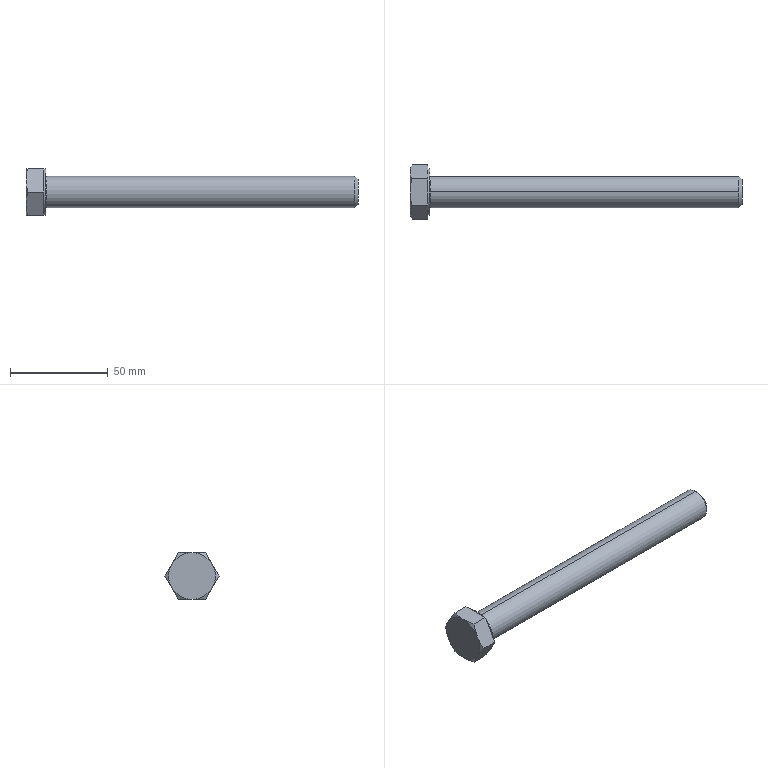Part | SolidWorks | features RevCut 4, Chamfer 1, Extrusion 1, Fillet 1, LPattern 1, Revolution 1 | 1 solid | 35 faces | box 170 x 27.713 x 24 mm | volume 37050 mm3 | plane 15 | cone 14 | cylinder 4 | torus 2 | commonest cylinder face diameters 16 x2 24 x2
STEP:
#1=CARTESIAN_POINT('',(10.6,0.,8.));
#2=VERTEX_POINT('',#1);
#3=CARTESIAN_POINT('',(10.6,0.,-8.));
#4=VERTEX_POINT('',#3);
#5=CARTESIAN_POINT('',(10.6,0.,0.));
#6=DIRECTION('',(1.,0.,0.));
#7=DIRECTION('',(0.,0.,-1.));
#8=AXIS2_PLACEMENT_3D('',#5,#6,#7);
#9=CIRCLE('',#8,8.);
#10=EDGE_CURVE('',#2,#4,#9,.T.);
#11=ORIENTED_EDGE('',*,*,#10,.F.);
#12=CARTESIAN_POINT('',(10.,0.,8.6));
#13=VERTEX_POINT('',#12);
#14=CARTESIAN_POINT('',(10.6,0.,8.6));
#15=DIRECTION('',(0.,1.,0.));
#16=DIRECTION('',(0.,0.,1.));
#17=AXIS2_PLACEMENT_3D('',#14,#15,#16);
#18=CIRCLE('',#17,0.6);
#19=EDGE_CURVE('',#2,#13,#18,.T.);
#20=ORIENTED_EDGE('',*,*,#19,.T.);
#21=CARTESIAN_POINT('',(10.,0.,-8.6));
#22=VERTEX_POINT('',#21);
#23=CARTESIAN_POINT('',(10.,0.,0.));
#24=DIRECTION('',(-1.,0.,0.));
#25=DIRECTION('',(0.,0.,-1.));
#26=AXIS2_PLACEMENT_3D('',#23,#24,#25);
#27=CIRCLE('',#26,8.6);
#28=EDGE_CURVE('',#22,#13,#27,.T.);
#29=ORIENTED_EDGE('',*,*,#28,.F.);
#30=CARTESIAN_POINT('',(10.6,0.,-8.6));
#31=DIRECTION('',(0.,-1.,0.));
#32=DIRECTION('',(0.,0.,-1.));
#33=AXIS2_PLACEMENT_3D('',#30,#31,#32);
#34=CIRCLE('',#33,0.6);
#35=EDGE_CURVE('',#4,#22,#34,.T.);
#36=ORIENTED_EDGE('',*,*,#35,.F.);
#37=EDGE_LOOP('',(#11,#20,#29,#36));
#38=FACE_OUTER_BOUND('',#37,.T.);
#39=CARTESIAN_POINT('',(10.6,0.,0.));
#40=DIRECTION('',(1.,0.,0.));
#41=DIRECTION('',(0.,0.,-1.));
#42=AXIS2_PLACEMENT_3D('',#39,#40,#41);
#43=TOROIDAL_SURFACE('',#42,8.6,0.6);
#44=ADVANCED_FACE('',(#38),#43,.F.);
#45=CARTESIAN_POINT('',(170.,0.,-6.4));
#46=VERTEX_POINT('',#45);
#47=CARTESIAN_POINT('',(170.,0.,6.4));
#48=VERTEX_POINT('',#47);
#49=CARTESIAN_POINT('',(170.,0.,0.));
#50=DIRECTION('',(1.,0.,0.));
#51=DIRECTION('',(0.,0.,1.));
#52=AXIS2_PLACEMENT_3D('',#49,#50,#51);
#53=CIRCLE('',#52,6.4);
#54=EDGE_CURVE('',#46,#48,#53,.T.);
#55=ORIENTED_EDGE('',*,*,#54,.F.);
#56=CARTESIAN_POINT('',(168.4,0.,-8.));
#57=VERTEX_POINT('',#56);
#58=CARTESIAN_POINT('',(168.4,0.,-8.));
#59=DIRECTION('',(-0.7071,0.,-0.7071));
#60=VECTOR('',#59,1000.);
#61=LINE('',#58,#60);
#62=EDGE_CURVE('',#46,#57,#61,.T.);
#63=ORIENTED_EDGE('',*,*,#62,.T.);
#64=CARTESIAN_POINT('',(168.4,0.,8.));
#65=VERTEX_POINT('',#64);
#66=CARTESIAN_POINT('',(168.4,0.,0.));
#67=DIRECTION('',(-1.,0.,0.));
#68=DIRECTION('',(0.,0.,1.));
#69=AXIS2_PLACEMENT_3D('',#66,#67,#68);
#70=CIRCLE('',#69,8.);
#71=EDGE_CURVE('',#65,#57,#70,.T.);
#72=ORIENTED_EDGE('',*,*,#71,.F.);
#73=CARTESIAN_POINT('',(168.4,0.,8.));
#74=DIRECTION('',(-0.7071,0.,0.7071));
#75=VECTOR('',#74,1000.);
#76=LINE('',#73,#75);
#77=EDGE_CURVE('',#48,#65,#76,.T.);
#78=ORIENTED_EDGE('',*,*,#77,.F.);
#79=EDGE_LOOP('',(#55,#63,#72,#78));
#80=FACE_OUTER_BOUND('',#79,.T.);
#81=CARTESIAN_POINT('',(168.4,0.,0.));
#82=DIRECTION('',(-1.,0.,0.));
#83=DIRECTION('',(0.,0.,1.));
#84=AXIS2_PLACEMENT_3D('',#81,#82,#83);
#85=CONICAL_SURFACE('',#84,8.,0.7854);
#86=ADVANCED_FACE('',(#80),#85,.T.);
#87=ORIENTED_EDGE('',*,*,#71,.T.);
#88=CARTESIAN_POINT('',(0.,0.,-8.));
#89=DIRECTION('',(-1.,0.,0.));
#90=VECTOR('',#89,1000.);
#91=LINE('',#88,#90);
#92=EDGE_CURVE('',#57,#4,#91,.T.);
#93=ORIENTED_EDGE('',*,*,#92,.T.);
#94=CARTESIAN_POINT('',(10.6,0.,0.));
#95=DIRECTION('',(1.,0.,0.));
#96=DIRECTION('',(0.,0.,-1.));
#97=AXIS2_PLACEMENT_3D('',#94,#95,#96);
#98=CIRCLE('',#97,8.);
#99=EDGE_CURVE('',#4,#2,#98,.T.);
#100=ORIENTED_EDGE('',*,*,#99,.T.);
#101=CARTESIAN_POINT('',(0.,0.,8.));
#102=DIRECTION('',(-1.,0.,0.));
#103=VECTOR('',#102,1000.);
#104=LINE('',#101,#103);
#105=EDGE_CURVE('',#65,#2,#104,.T.);
#106=ORIENTED_EDGE('',*,*,#105,.F.);
#107=EDGE_LOOP('',(#87,#93,#100,#106));
#108=FACE_OUTER_BOUND('',#107,.T.);
#109=CARTESIAN_POINT('',(0.,0.,0.));
#110=DIRECTION('',(-1.,0.,0.));
#111=DIRECTION('',(0.,0.,1.));
#112=AXIS2_PLACEMENT_3D('',#109,#110,#111);
#113=CYLINDRICAL_SURFACE('',#112,8.);
#114=ADVANCED_FACE('',(#108),#113,.T.);
#115=CARTESIAN_POINT('',(10.,0.,-12.));
#116=VERTEX_POINT('',#115);
#117=CARTESIAN_POINT('',(10.,0.,12.));
#118=VERTEX_POINT('',#117);
#119=CARTESIAN_POINT('',(10.,0.,0.));
#120=DIRECTION('',(1.,0.,0.));
#121=DIRECTION('',(0.,0.,-1.));
#122=AXIS2_PLACEMENT_3D('',#119,#120,#121);
#123=CIRCLE('',#122,12.);
#124=EDGE_CURVE('',#116,#118,#123,.T.);
#125=ORIENTED_EDGE('',*,*,#124,.F.);
#126=CARTESIAN_POINT('',(9.2,0.,-12.));
#127=VERTEX_POINT('',#126);
#128=CARTESIAN_POINT('',(0.,0.,-12.));
#129=DIRECTION('',(-1.,0.,0.));
#130=VECTOR('',#129,1000.);
#131=LINE('',#128,#130);
#132=EDGE_CURVE('',#116,#127,#131,.T.);
#133=ORIENTED_EDGE('',*,*,#132,.T.);
#134=CARTESIAN_POINT('',(9.2,10.392,-6.));
#135=VERTEX_POINT('',#134);
#136=CARTESIAN_POINT('',(9.2,0.,0.));
#137=DIRECTION('',(-1.,0.,0.));
#138=DIRECTION('',(0.,0.,1.));
#139=AXIS2_PLACEMENT_3D('',#136,#137,#138);
#140=CIRCLE('',#139,12.);
#141=EDGE_CURVE('',#135,#127,#140,.T.);
#142=ORIENTED_EDGE('',*,*,#141,.F.);
#143=CARTESIAN_POINT('',(9.2,10.392,6.));
#144=VERTEX_POINT('',#143);
#145=CARTESIAN_POINT('',(9.2,0.,0.));
#146=DIRECTION('',(-1.,0.,0.));
#147=DIRECTION('',(0.,0.,1.));
#148=AXIS2_PLACEMENT_3D('',#145,#146,#147);
#149=CIRCLE('',#148,12.);
#150=EDGE_CURVE('',#144,#135,#149,.T.);
#151=ORIENTED_EDGE('',*,*,#150,.F.);
#152=CARTESIAN_POINT('',(9.2,0.,12.));
#153=VERTEX_POINT('',#152);
#154=CARTESIAN_POINT('',(9.2,0.,0.));
#155=DIRECTION('',(-1.,0.,0.));
#156=DIRECTION('',(0.,0.,1.));
#157=AXIS2_PLACEMENT_3D('',#154,#155,#156);
#158=CIRCLE('',#157,12.);
#159=EDGE_CURVE('',#153,#144,#158,.T.);
#160=ORIENTED_EDGE('',*,*,#159,.F.);
#161=CARTESIAN_POINT('',(0.,0.,12.));
#162=DIRECTION('',(-1.,0.,0.));
#163=VECTOR('',#162,1000.);
#164=LINE('',#161,#163);
#165=EDGE_CURVE('',#118,#153,#164,.T.);
#166=ORIENTED_EDGE('',*,*,#165,.F.);
#167=EDGE_LOOP('',(#125,#133,#142,#151,#160,#166));
#168=FACE_OUTER_BOUND('',#167,.T.);
#169=CARTESIAN_POINT('',(0.,0.,0.));
#170=DIRECTION('',(-1.,0.,0.));
#171=DIRECTION('',(0.,0.,1.));
#172=AXIS2_PLACEMENT_3D('',#169,#170,#171);
#173=CYLINDRICAL_SURFACE('',#172,12.);
#174=ADVANCED_FACE('',(#168),#173,.T.);
#175=CARTESIAN_POINT('',(9.2,7.427,-11.136));
#176=VERTEX_POINT('',#175);
#177=CARTESIAN_POINT('',(9.2,6.928,-12.));
#178=DIRECTION('',(0.,0.5,0.866));
#179=VECTOR('',#178,1000.);
#180=LINE('',#177,#179);
#181=EDGE_CURVE('',#176,#135,#180,.T.);
#182=ORIENTED_EDGE('',*,*,#181,.F.);
#183=CARTESIAN_POINT('',(8.928,6.928,-12.));
#184=VERTEX_POINT('',#183);
#185=CARTESIAN_POINT('',(8.928,6.928,-12.));
#186=CARTESIAN_POINT('',(9.024,7.094,-11.713));
#187=CARTESIAN_POINT('',(9.115,7.26,-11.425));
#188=CARTESIAN_POINT('',(9.2,7.427,-11.136));
#189=B_SPLINE_CURVE_WITH_KNOTS('',3,(#185,#186,#187,#188),.UNSPECIFIED.,.F.,.F.,(4,4),(0.000000238,0.001026),.UNSPECIFIED.);
#190=EDGE_CURVE('',#184,#176,#189,.T.);
#191=ORIENTED_EDGE('',*,*,#190,.F.);
#192=CARTESIAN_POINT('',(1.072,6.928,-12.));
#193=VERTEX_POINT('',#192);
#194=CARTESIAN_POINT('',(10.,6.928,-12.));
#195=DIRECTION('',(-1.,0.,0.));
#196=VECTOR('',#195,1000.);
#197=LINE('',#194,#196);
#198=EDGE_CURVE('',#184,#193,#197,.T.);
#199=ORIENTED_EDGE('',*,*,#198,.T.);
#200=CARTESIAN_POINT('',(0.,10.392,-6.));
#201=VERTEX_POINT('',#200);
#202=CARTESIAN_POINT('',(0.,10.392,-6.));
#203=CARTESIAN_POINT('',(0.,10.098,-6.509));
#204=CARTESIAN_POINT('',(0.02533,9.803,-7.021));
#205=CARTESIAN_POINT('',(0.1234,9.219,-8.033));
#206=CARTESIAN_POINT('',(0.196,8.929,-8.535));
#207=CARTESIAN_POINT('',(0.476,8.063,-10.034));
#208=CARTESIAN_POINT('',(0.7454,7.493,-11.021));
#209=CARTESIAN_POINT('',(1.072,6.928,-12.));
#210=B_SPLINE_CURVE_WITH_KNOTS('',3,(#202,#203,#204,#205,#206,#207,#208,#209),.UNSPECIFIED.,.F.,.F.,(4,2,2,4),(0.00701,0.008756,0.0105,0.01399),.UNSPECIFIED.);
#211=EDGE_CURVE('',#201,#193,#210,.T.);
#212=ORIENTED_EDGE('',*,*,#211,.F.);
#213=CARTESIAN_POINT('',(1.072,13.856,0.));
#214=VERTEX_POINT('',#213);
#215=CARTESIAN_POINT('',(1.072,13.856,0.));
#216=CARTESIAN_POINT('',(0.7446,13.29,-0.9815));
#217=CARTESIAN_POINT('',(0.4751,12.719,-1.97));
#218=CARTESIAN_POINT('',(0.1021,11.565,-3.968));
#219=CARTESIAN_POINT('',(0.,10.982,-4.978));
#220=CARTESIAN_POINT('',(0.,10.392,-6.));
#221=B_SPLINE_CURVE_WITH_KNOTS('',3,(#215,#216,#217,#218,#219,#220),.UNSPECIFIED.,.F.,.F.,(4,2,4),(0.000000238,0.003505,0.00701),.UNSPECIFIED.);
#222=EDGE_CURVE('',#214,#201,#221,.T.);
#223=ORIENTED_EDGE('',*,*,#222,.F.);
#224=CARTESIAN_POINT('',(8.928,13.856,0.));
#225=VERTEX_POINT('',#224);
#226=CARTESIAN_POINT('',(10.,13.856,0.));
#227=DIRECTION('',(-1.,0.,0.));
#228=VECTOR('',#227,1000.);
#229=LINE('',#226,#228);
#230=EDGE_CURVE('',#225,#214,#229,.T.);
#231=ORIENTED_EDGE('',*,*,#230,.F.);
#232=CARTESIAN_POINT('',(9.2,13.358,-0.8637));
#233=VERTEX_POINT('',#232);
#234=CARTESIAN_POINT('',(9.2,13.358,-0.8637));
#235=CARTESIAN_POINT('',(9.115,13.524,-0.575));
#236=CARTESIAN_POINT('',(9.024,13.691,-0.2872));
#237=CARTESIAN_POINT('',(8.928,13.856,0.));
#238=B_SPLINE_CURVE_WITH_KNOTS('',3,(#234,#235,#236,#237),.UNSPECIFIED.,.F.,.F.,(4,4),(0.01297,0.01399),.UNSPECIFIED.);
#239=EDGE_CURVE('',#233,#225,#238,.T.);
#240=ORIENTED_EDGE('',*,*,#239,.F.);
#241=CARTESIAN_POINT('',(9.2,6.928,-12.));
#242=DIRECTION('',(0.,0.5,0.866));
#243=VECTOR('',#242,1000.);
#244=LINE('',#241,#243);
#245=EDGE_CURVE('',#135,#233,#244,.T.);
#246=ORIENTED_EDGE('',*,*,#245,.F.);
#247=EDGE_LOOP('',(#182,#191,#199,#212,#223,#231,#240,#246));
#248=FACE_OUTER_BOUND('',#247,.T.);
#249=CARTESIAN_POINT('',(10.,6.928,-12.));
#250=DIRECTION('',(0.,-0.866,0.5));
#251=DIRECTION('',(0.,-0.5,-0.866));
#252=AXIS2_PLACEMENT_3D('',#249,#250,#251);
#253=PLANE('',#252);
#254=ADVANCED_FACE('',(#248),#253,.F.);
#255=CARTESIAN_POINT('',(9.2,13.358,0.8637));
#256=VERTEX_POINT('',#255);
#257=CARTESIAN_POINT('',(9.2,13.856,0.));
#258=DIRECTION('',(0.,-0.5,0.866));
#259=VECTOR('',#258,1000.);
#260=LINE('',#257,#259);
#261=EDGE_CURVE('',#256,#144,#260,.T.);
#262=ORIENTED_EDGE('',*,*,#261,.F.);
#263=CARTESIAN_POINT('',(8.928,13.856,0.));
#264=CARTESIAN_POINT('',(9.024,13.691,0.2873));
#265=CARTESIAN_POINT('',(9.115,13.524,0.5751));
#266=CARTESIAN_POINT('',(9.2,13.358,0.8637));
#267=B_SPLINE_CURVE_WITH_KNOTS('',3,(#263,#264,#265,#266),.UNSPECIFIED.,.F.,.F.,(4,4),(0.000000238,0.001026),.UNSPECIFIED.);
#268=EDGE_CURVE('',#225,#256,#267,.T.);
#269=ORIENTED_EDGE('',*,*,#268,.F.);
#270=ORIENTED_EDGE('',*,*,#230,.T.);
#271=CARTESIAN_POINT('',(0.,10.392,6.));
#272=VERTEX_POINT('',#271);
#273=CARTESIAN_POINT('',(0.,10.392,6.));
#274=CARTESIAN_POINT('',(0.,10.686,5.491));
#275=CARTESIAN_POINT('',(0.02533,10.982,4.979));
#276=CARTESIAN_POINT('',(0.1234,11.566,3.967));
#277=CARTESIAN_POINT('',(0.196,11.856,3.465));
#278=CARTESIAN_POINT('',(0.476,12.721,1.966));
#279=CARTESIAN_POINT('',(0.7454,13.291,0.9791));
#280=CARTESIAN_POINT('',(1.072,13.856,0.));
#281=B_SPLINE_CURVE_WITH_KNOTS('',3,(#273,#274,#275,#276,#277,#278,#279,#280),.UNSPECIFIED.,.F.,.F.,(4,2,2,4),(0.00701,0.008756,0.0105,0.01399),.UNSPECIFIED.);
#282=EDGE_CURVE('',#272,#214,#281,.T.);
#283=ORIENTED_EDGE('',*,*,#282,.F.);
#284=CARTESIAN_POINT('',(1.072,6.928,12.));
#285=VERTEX_POINT('',#284);
#286=CARTESIAN_POINT('',(1.072,6.928,12.));
#287=CARTESIAN_POINT('',(0.7446,7.495,11.018));
#288=CARTESIAN_POINT('',(0.4751,8.066,10.03));
#289=CARTESIAN_POINT('',(0.1021,9.219,8.032));
#290=CARTESIAN_POINT('',(0.,9.802,7.022));
#291=CARTESIAN_POINT('',(0.,10.392,6.));
#292=B_SPLINE_CURVE_WITH_KNOTS('',3,(#286,#287,#288,#289,#290,#291),.UNSPECIFIED.,.F.,.F.,(4,2,4),(0.000000238,0.003505,0.00701),.UNSPECIFIED.);
#293=EDGE_CURVE('',#285,#272,#292,.T.);
#294=ORIENTED_EDGE('',*,*,#293,.F.);
#295=CARTESIAN_POINT('',(8.928,6.928,12.));
#296=VERTEX_POINT('',#295);
#297=CARTESIAN_POINT('',(10.,6.928,12.));
#298=DIRECTION('',(-1.,0.,0.));
#299=VECTOR('',#298,1000.);
#300=LINE('',#297,#299);
#301=EDGE_CURVE('',#296,#285,#300,.T.);
#302=ORIENTED_EDGE('',*,*,#301,.F.);
#303=CARTESIAN_POINT('',(9.2,7.427,11.136));
#304=VERTEX_POINT('',#303);
#305=CARTESIAN_POINT('',(9.2,7.427,11.136));
#306=CARTESIAN_POINT('',(9.115,7.26,11.425));
#307=CARTESIAN_POINT('',(9.024,7.094,11.713));
#308=CARTESIAN_POINT('',(8.928,6.928,12.));
#309=B_SPLINE_CURVE_WITH_KNOTS('',3,(#305,#306,#307,#308),.UNSPECIFIED.,.F.,.F.,(4,4),(0.01297,0.01399),.UNSPECIFIED.);
#310=EDGE_CURVE('',#304,#296,#309,.T.);
#311=ORIENTED_EDGE('',*,*,#310,.F.);
#312=CARTESIAN_POINT('',(9.2,13.856,0.));
#313=DIRECTION('',(0.,-0.5,0.866));
#314=VECTOR('',#313,1000.);
#315=LINE('',#312,#314);
#316=EDGE_CURVE('',#144,#304,#315,.T.);
#317=ORIENTED_EDGE('',*,*,#316,.F.);
#318=EDGE_LOOP('',(#262,#269,#270,#283,#294,#302,#311,#317));
#319=FACE_OUTER_BOUND('',#318,.T.);
#320=CARTESIAN_POINT('',(10.,13.856,0.));
#321=DIRECTION('',(0.,-0.866,-0.5));
#322=DIRECTION('',(0.,0.5,-0.866));
#323=AXIS2_PLACEMENT_3D('',#320,#321,#322);
#324=PLANE('',#323);
#325=ADVANCED_FACE('',(#319),#324,.F.);
#326=CARTESIAN_POINT('',(9.2,5.931,12.));
#327=VERTEX_POINT('',#326);
#328=CARTESIAN_POINT('',(9.2,6.928,12.));
#329=DIRECTION('',(0.,-1.,0.));
#330=VECTOR('',#329,1000.);
#331=LINE('',#328,#330);
#332=EDGE_CURVE('',#327,#153,#331,.T.);
#333=ORIENTED_EDGE('',*,*,#332,.F.);
#334=CARTESIAN_POINT('',(8.928,6.928,12.));
#335=CARTESIAN_POINT('',(9.024,6.597,12.));
#336=CARTESIAN_POINT('',(9.115,6.265,12.));
#337=CARTESIAN_POINT('',(9.2,5.931,12.));
#338=B_SPLINE_CURVE_WITH_KNOTS('',3,(#334,#335,#336,#337),.UNSPECIFIED.,.F.,.F.,(4,4),(0.03236,0.0334),.UNSPECIFIED.);
#339=EDGE_CURVE('',#296,#327,#338,.T.);
#340=ORIENTED_EDGE('',*,*,#339,.F.);
#341=ORIENTED_EDGE('',*,*,#301,.T.);
#342=CARTESIAN_POINT('',(0.,0.,12.));
#343=VERTEX_POINT('',#342);
#344=CARTESIAN_POINT('',(0.,0.,12.));
#345=CARTESIAN_POINT('',(0.,0.5865,12.));
#346=CARTESIAN_POINT('',(0.02506,1.176,12.));
#347=CARTESIAN_POINT('',(0.1242,2.355,12.));
#348=CARTESIAN_POINT('',(0.1975,2.939,12.));
#349=CARTESIAN_POINT('',(0.4791,4.673,12.));
#350=CARTESIAN_POINT('',(0.7483,5.808,12.));
#351=CARTESIAN_POINT('',(1.072,6.928,12.));
#352=B_SPLINE_CURVE_WITH_KNOTS('',3,(#344,#345,#346,#347,#348,#349,#350,#351),.UNSPECIFIED.,.F.,.F.,(4,2,2,4),(0.01982,0.02158,0.02333,0.02684),.UNSPECIFIED.);
#353=EDGE_CURVE('',#343,#285,#352,.T.);
#354=ORIENTED_EDGE('',*,*,#353,.F.);
#355=CARTESIAN_POINT('',(1.072,-6.928,12.));
#356=VERTEX_POINT('',#355);
#357=CARTESIAN_POINT('',(1.072,-6.928,12.));
#358=CARTESIAN_POINT('',(0.7461,-5.8,12.));
#359=CARTESIAN_POINT('',(0.4736,-4.647,12.));
#360=CARTESIAN_POINT('',(0.1008,-2.335,12.));
#361=CARTESIAN_POINT('',(0.,-1.172,12.));
#362=CARTESIAN_POINT('',(0.,0.,12.));
#363=B_SPLINE_CURVE_WITH_KNOTS('',3,(#357,#358,#359,#360,#361,#362),.UNSPECIFIED.,.F.,.F.,(4,2,4),(0.01281,0.01632,0.01982),.UNSPECIFIED.);
#364=EDGE_CURVE('',#356,#343,#363,.T.);
#365=ORIENTED_EDGE('',*,*,#364,.F.);
#366=CARTESIAN_POINT('',(8.928,-6.928,12.));
#367=VERTEX_POINT('',#366);
#368=CARTESIAN_POINT('',(10.,-6.928,12.));
#369=DIRECTION('',(-1.,0.,0.));
#370=VECTOR('',#369,1000.);
#371=LINE('',#368,#370);
#372=EDGE_CURVE('',#367,#356,#371,.T.);
#373=ORIENTED_EDGE('',*,*,#372,.F.);
#374=CARTESIAN_POINT('',(9.2,-5.931,12.));
#375=VERTEX_POINT('',#374);
#376=CARTESIAN_POINT('',(9.2,-5.931,12.));
#377=CARTESIAN_POINT('',(9.114,-6.265,12.));
#378=CARTESIAN_POINT('',(9.024,-6.598,12.));
#379=CARTESIAN_POINT('',(8.928,-6.928,12.));
#380=B_SPLINE_CURVE_WITH_KNOTS('',3,(#376,#377,#378,#379),.UNSPECIFIED.,.F.,.F.,(4,4),(0.04537,0.0464),.UNSPECIFIED.);
#381=EDGE_CURVE('',#375,#367,#380,.T.);
#382=ORIENTED_EDGE('',*,*,#381,.F.);
#383=CARTESIAN_POINT('',(9.2,6.928,12.));
#384=DIRECTION('',(0.,-1.,0.));
#385=VECTOR('',#384,1000.);
#386=LINE('',#383,#385);
#387=EDGE_CURVE('',#153,#375,#386,.T.);
#388=ORIENTED_EDGE('',*,*,#387,.F.);
#389=EDGE_LOOP('',(#333,#340,#341,#354,#365,#373,#382,#388));
#390=FACE_OUTER_BOUND('',#389,.T.);
#391=CARTESIAN_POINT('',(10.,6.928,12.));
#392=DIRECTION('',(0.,0.,-1.));
#393=DIRECTION('',(-1.,0.,0.));
#394=AXIS2_PLACEMENT_3D('',#391,#392,#393);
#395=PLANE('',#394);
#396=ADVANCED_FACE('',(#390),#395,.F.);
#397=CARTESIAN_POINT('',(9.2,-7.427,11.136));
#398=VERTEX_POINT('',#397);
#399=CARTESIAN_POINT('',(9.2,-10.392,6.));
#400=VERTEX_POINT('',#399);
#401=CARTESIAN_POINT('',(9.2,-13.856,0.));
#402=DIRECTION('',(0.,-0.5,-0.866));
#403=VECTOR('',#402,1000.);
#404=LINE('',#401,#403);
#405=EDGE_CURVE('',#398,#400,#404,.T.);
#406=ORIENTED_EDGE('',*,*,#405,.F.);
#407=CARTESIAN_POINT('',(8.928,-6.928,12.));
#408=CARTESIAN_POINT('',(9.024,-7.094,11.713));
#409=CARTESIAN_POINT('',(9.115,-7.26,11.425));
#410=CARTESIAN_POINT('',(9.2,-7.427,11.136));
#411=B_SPLINE_CURVE_WITH_KNOTS('',3,(#407,#408,#409,#410),.UNSPECIFIED.,.F.,.F.,(4,4),(0.000000238,0.001026),.UNSPECIFIED.);
#412=EDGE_CURVE('',#367,#398,#411,.T.);
#413=ORIENTED_EDGE('',*,*,#412,.F.);
#414=ORIENTED_EDGE('',*,*,#372,.T.);
#415=CARTESIAN_POINT('',(0.,-10.392,6.));
#416=VERTEX_POINT('',#415);
#417=CARTESIAN_POINT('',(0.,-10.392,6.));
#418=CARTESIAN_POINT('',(0.,-10.098,6.509));
#419=CARTESIAN_POINT('',(0.02533,-9.803,7.021));
#420=CARTESIAN_POINT('',(0.1234,-9.219,8.033));
#421=CARTESIAN_POINT('',(0.196,-8.929,8.535));
#422=CARTESIAN_POINT('',(0.476,-8.063,10.034));
#423=CARTESIAN_POINT('',(0.7454,-7.493,11.021));
#424=CARTESIAN_POINT('',(1.072,-6.928,12.));
#425=B_SPLINE_CURVE_WITH_KNOTS('',3,(#417,#418,#419,#420,#421,#422,#423,#424),.UNSPECIFIED.,.F.,.F.,(4,2,2,4),(0.00701,0.008756,0.0105,0.01399),.UNSPECIFIED.);
#426=EDGE_CURVE('',#416,#356,#425,.T.);
#427=ORIENTED_EDGE('',*,*,#426,.F.);
#428=CARTESIAN_POINT('',(1.072,-13.856,0.));
#429=VERTEX_POINT('',#428);
#430=CARTESIAN_POINT('',(1.072,-13.856,0.));
#431=CARTESIAN_POINT('',(0.7446,-13.29,0.9815));
#432=CARTESIAN_POINT('',(0.4751,-12.719,1.97));
#433=CARTESIAN_POINT('',(0.1021,-11.565,3.968));
#434=CARTESIAN_POINT('',(0.,-10.982,4.978));
#435=CARTESIAN_POINT('',(0.,-10.392,6.));
#436=B_SPLINE_CURVE_WITH_KNOTS('',3,(#430,#431,#432,#433,#434,#435),.UNSPECIFIED.,.F.,.F.,(4,2,4),(0.000000238,0.003505,0.00701),.UNSPECIFIED.);
#437=EDGE_CURVE('',#429,#416,#436,.T.);
#438=ORIENTED_EDGE('',*,*,#437,.F.);
#439=CARTESIAN_POINT('',(8.928,-13.856,0.));
#440=VERTEX_POINT('',#439);
#441=CARTESIAN_POINT('',(10.,-13.856,0.));
#442=DIRECTION('',(-1.,0.,0.));
#443=VECTOR('',#442,1000.);
#444=LINE('',#441,#443);
#445=EDGE_CURVE('',#440,#429,#444,.T.);
#446=ORIENTED_EDGE('',*,*,#445,.F.);
#447=CARTESIAN_POINT('',(9.2,-13.358,0.8637));
#448=VERTEX_POINT('',#447);
#449=CARTESIAN_POINT('',(9.2,-13.358,0.8637));
#450=CARTESIAN_POINT('',(9.115,-13.524,0.575));
#451=CARTESIAN_POINT('',(9.024,-13.691,0.2872));
#452=CARTESIAN_POINT('',(8.928,-13.856,0.));
#453=B_SPLINE_CURVE_WITH_KNOTS('',3,(#449,#450,#451,#452),.UNSPECIFIED.,.F.,.F.,(4,4),(0.01297,0.01399),.UNSPECIFIED.);
#454=EDGE_CURVE('',#448,#440,#453,.T.);
#455=ORIENTED_EDGE('',*,*,#454,.F.);
#456=CARTESIAN_POINT('',(9.2,-13.856,0.));
#457=DIRECTION('',(0.,-0.5,-0.866));
#458=VECTOR('',#457,1000.);
#459=LINE('',#456,#458);
#460=EDGE_CURVE('',#400,#448,#459,.T.);
#461=ORIENTED_EDGE('',*,*,#460,.F.);
#462=EDGE_LOOP('',(#406,#413,#414,#427,#438,#446,#455,#461));
#463=FACE_OUTER_BOUND('',#462,.T.);
#464=CARTESIAN_POINT('',(10.,-13.856,0.));
#465=DIRECTION('',(0.,0.866,-0.5));
#466=DIRECTION('',(0.,0.5,0.866));
#467=AXIS2_PLACEMENT_3D('',#464,#465,#466);
#468=PLANE('',#467);
#469=ADVANCED_FACE('',(#463),#468,.F.);
#470=CARTESIAN_POINT('',(9.2,-13.358,-0.8637));
#471=VERTEX_POINT('',#470);
#472=CARTESIAN_POINT('',(9.2,-10.392,-6.));
#473=VERTEX_POINT('',#472);
#474=CARTESIAN_POINT('',(9.2,-6.928,-12.));
#475=DIRECTION('',(0.,0.5,-0.866));
#476=VECTOR('',#475,1000.);
#477=LINE('',#474,#476);
#478=EDGE_CURVE('',#471,#473,#477,.T.);
#479=ORIENTED_EDGE('',*,*,#478,.F.);
#480=CARTESIAN_POINT('',(8.928,-13.856,0.));
#481=CARTESIAN_POINT('',(9.024,-13.691,-0.2873));
#482=CARTESIAN_POINT('',(9.115,-13.524,-0.5751));
#483=CARTESIAN_POINT('',(9.2,-13.358,-0.8637));
#484=B_SPLINE_CURVE_WITH_KNOTS('',3,(#480,#481,#482,#483),.UNSPECIFIED.,.F.,.F.,(4,4),(0.000000238,0.001026),.UNSPECIFIED.);
#485=EDGE_CURVE('',#440,#471,#484,.T.);
#486=ORIENTED_EDGE('',*,*,#485,.F.);
#487=ORIENTED_EDGE('',*,*,#445,.T.);
#488=CARTESIAN_POINT('',(0.,-10.392,-6.));
#489=VERTEX_POINT('',#488);
#490=CARTESIAN_POINT('',(0.,-10.392,-6.));
#491=CARTESIAN_POINT('',(0.,-10.686,-5.491));
#492=CARTESIAN_POINT('',(0.02533,-10.982,-4.979));
#493=CARTESIAN_POINT('',(0.1234,-11.566,-3.967));
#494=CARTESIAN_POINT('',(0.196,-11.856,-3.465));
#495=CARTESIAN_POINT('',(0.476,-12.721,-1.966));
#496=CARTESIAN_POINT('',(0.7454,-13.291,-0.9791));
#497=CARTESIAN_POINT('',(1.072,-13.856,0.));
#498=B_SPLINE_CURVE_WITH_KNOTS('',3,(#490,#491,#492,#493,#494,#495,#496,#497),.UNSPECIFIED.,.F.,.F.,(4,2,2,4),(0.00701,0.008756,0.0105,0.01399),.UNSPECIFIED.);
#499=EDGE_CURVE('',#489,#429,#498,.T.);
#500=ORIENTED_EDGE('',*,*,#499,.F.);
#501=CARTESIAN_POINT('',(1.072,-6.928,-12.));
#502=VERTEX_POINT('',#501);
#503=CARTESIAN_POINT('',(1.072,-6.928,-12.));
#504=CARTESIAN_POINT('',(0.7446,-7.495,-11.018));
#505=CARTESIAN_POINT('',(0.4751,-8.066,-10.03));
#506=CARTESIAN_POINT('',(0.1021,-9.219,-8.032));
#507=CARTESIAN_POINT('',(0.,-9.802,-7.022));
#508=CARTESIAN_POINT('',(0.,-10.392,-6.));
#509=B_SPLINE_CURVE_WITH_KNOTS('',3,(#503,#504,#505,#506,#507,#508),.UNSPECIFIED.,.F.,.F.,(4,2,4),(0.000000238,0.003505,0.00701),.UNSPECIFIED.);
#510=EDGE_CURVE('',#502,#489,#509,.T.);
#511=ORIENTED_EDGE('',*,*,#510,.F.);
#512=CARTESIAN_POINT('',(8.928,-6.928,-12.));
#513=VERTEX_POINT('',#512);
#514=CARTESIAN_POINT('',(10.,-6.928,-12.));
#515=DIRECTION('',(-1.,0.,0.));
#516=VECTOR('',#515,1000.);
#517=LINE('',#514,#516);
#518=EDGE_CURVE('',#513,#502,#517,.T.);
#519=ORIENTED_EDGE('',*,*,#518,.F.);
#520=CARTESIAN_POINT('',(9.2,-7.427,-11.136));
#521=VERTEX_POINT('',#520);
#522=CARTESIAN_POINT('',(9.2,-7.427,-11.136));
#523=CARTESIAN_POINT('',(9.115,-7.26,-11.425));
#524=CARTESIAN_POINT('',(9.024,-7.094,-11.713));
#525=CARTESIAN_POINT('',(8.928,-6.928,-12.));
#526=B_SPLINE_CURVE_WITH_KNOTS('',3,(#522,#523,#524,#525),.UNSPECIFIED.,.F.,.F.,(4,4),(0.01297,0.01399),.UNSPECIFIED.);
#527=EDGE_CURVE('',#521,#513,#526,.T.);
#528=ORIENTED_EDGE('',*,*,#527,.F.);
#529=CARTESIAN_POINT('',(9.2,-6.928,-12.));
#530=DIRECTION('',(0.,0.5,-0.866));
#531=VECTOR('',#530,1000.);
#532=LINE('',#529,#531);
#533=EDGE_CURVE('',#473,#521,#532,.T.);
#534=ORIENTED_EDGE('',*,*,#533,.F.);
#535=EDGE_LOOP('',(#479,#486,#487,#500,#511,#519,#528,#534));
#536=FACE_OUTER_BOUND('',#535,.T.);
#537=CARTESIAN_POINT('',(10.,-6.928,-12.));
#538=DIRECTION('',(0.,0.866,0.5));
#539=DIRECTION('',(0.,-0.5,0.866));
#540=AXIS2_PLACEMENT_3D('',#537,#538,#539);
#541=PLANE('',#540);
#542=ADVANCED_FACE('',(#536),#541,.F.);
#543=CARTESIAN_POINT('',(9.2,-5.931,-12.));
#544=VERTEX_POINT('',#543);
#545=CARTESIAN_POINT('',(9.2,6.928,-12.));
#546=DIRECTION('',(0.,1.,0.));
#547=VECTOR('',#546,1000.);
#548=LINE('',#545,#547);
#549=EDGE_CURVE('',#544,#127,#548,.T.);
#550=ORIENTED_EDGE('',*,*,#549,.F.);
#551=CARTESIAN_POINT('',(8.928,-6.928,-12.));
#552=CARTESIAN_POINT('',(9.024,-6.598,-12.));
#553=CARTESIAN_POINT('',(9.114,-6.265,-12.));
#554=CARTESIAN_POINT('',(9.2,-5.931,-12.));
#555=B_SPLINE_CURVE_WITH_KNOTS('',3,(#551,#552,#553,#554),.UNSPECIFIED.,.F.,.F.,(4,4),(0.01281,0.01384),.UNSPECIFIED.);
#556=EDGE_CURVE('',#513,#544,#555,.T.);
#557=ORIENTED_EDGE('',*,*,#556,.F.);
#558=ORIENTED_EDGE('',*,*,#518,.T.);
#559=CARTESIAN_POINT('',(0.,0.,-12.));
#560=VERTEX_POINT('',#559);
#561=CARTESIAN_POINT('',(0.,0.,-12.));
#562=CARTESIAN_POINT('',(0.,-1.172,-12.));
#563=CARTESIAN_POINT('',(0.1008,-2.335,-12.));
#564=CARTESIAN_POINT('',(0.4736,-4.647,-12.));
#565=CARTESIAN_POINT('',(0.7461,-5.8,-12.));
#566=CARTESIAN_POINT('',(1.072,-6.928,-12.));
#567=B_SPLINE_CURVE_WITH_KNOTS('',3,(#561,#562,#563,#564,#565,#566),.UNSPECIFIED.,.F.,.F.,(4,2,4),(0.03938,0.04289,0.0464),.UNSPECIFIED.);
#568=EDGE_CURVE('',#560,#502,#567,.T.);
#569=ORIENTED_EDGE('',*,*,#568,.F.);
#570=CARTESIAN_POINT('',(1.072,6.928,-12.));
#571=CARTESIAN_POINT('',(0.7483,5.808,-12.));
#572=CARTESIAN_POINT('',(0.4791,4.673,-12.));
#573=CARTESIAN_POINT('',(0.1975,2.939,-12.));
#574=CARTESIAN_POINT('',(0.1242,2.355,-12.));
#575=CARTESIAN_POINT('',(0.02506,1.176,-12.));
#576=CARTESIAN_POINT('',(0.,0.5865,-12.));
#577=CARTESIAN_POINT('',(0.,0.,-12.));
#578=B_SPLINE_CURVE_WITH_KNOTS('',3,(#570,#571,#572,#573,#574,#575,#576,#577),.UNSPECIFIED.,.F.,.F.,(4,2,2,4),(0.03236,0.03587,0.03763,0.03938),.UNSPECIFIED.);
#579=EDGE_CURVE('',#193,#560,#578,.T.);
#580=ORIENTED_EDGE('',*,*,#579,.F.);
#581=ORIENTED_EDGE('',*,*,#198,.F.);
#582=CARTESIAN_POINT('',(9.2,5.931,-12.));
#583=VERTEX_POINT('',#582);
#584=CARTESIAN_POINT('',(9.2,5.931,-12.));
#585=CARTESIAN_POINT('',(9.115,6.265,-12.));
#586=CARTESIAN_POINT('',(9.024,6.597,-12.));
#587=CARTESIAN_POINT('',(8.928,6.928,-12.));
#588=B_SPLINE_CURVE_WITH_KNOTS('',3,(#584,#585,#586,#587),.UNSPECIFIED.,.F.,.F.,(4,4),(0.0258,0.02684),.UNSPECIFIED.);
#589=EDGE_CURVE('',#583,#184,#588,.T.);
#590=ORIENTED_EDGE('',*,*,#589,.F.);
#591=CARTESIAN_POINT('',(9.2,6.928,-12.));
#592=DIRECTION('',(0.,1.,0.));
#593=VECTOR('',#592,1000.);
#594=LINE('',#591,#593);
#595=EDGE_CURVE('',#127,#583,#594,.T.);
#596=ORIENTED_EDGE('',*,*,#595,.F.);
#597=EDGE_LOOP('',(#550,#557,#558,#569,#580,#581,#590,#596));
#598=FACE_OUTER_BOUND('',#597,.T.);
#599=CARTESIAN_POINT('',(10.,6.928,-12.));
#600=DIRECTION('',(0.,0.,1.));
#601=DIRECTION('',(0.,-1.,0.));
#602=AXIS2_PLACEMENT_3D('',#599,#600,#601);
#603=PLANE('',#602);
#604=ADVANCED_FACE('',(#598),#603,.F.);
#605=ORIENTED_EDGE('',*,*,#556,.T.);
#606=CARTESIAN_POINT('',(9.2,0.,0.));
#607=DIRECTION('',(-1.,0.,0.));
#608=DIRECTION('',(0.,0.,-1.));
#609=AXIS2_PLACEMENT_3D('',#606,#607,#608);
#610=CIRCLE('',#609,13.386);
#611=EDGE_CURVE('',#544,#521,#610,.T.);
#612=ORIENTED_EDGE('',*,*,#611,.T.);
#613=ORIENTED_EDGE('',*,*,#527,.T.);
#614=EDGE_LOOP('',(#605,#612,#613));
#615=FACE_OUTER_BOUND('',#614,.T.);
#616=CARTESIAN_POINT('',(6.041,0.,0.));
#617=DIRECTION('',(-1.,0.,0.));
#618=DIRECTION('',(0.,0.,1.));
#619=AXIS2_PLACEMENT_3D('',#616,#617,#618);
#620=CONICAL_SURFACE('',#619,18.856,1.047);
#621=ADVANCED_FACE('',(#615),#620,.T.);
#622=ORIENTED_EDGE('',*,*,#485,.T.);
#623=CARTESIAN_POINT('',(9.2,0.,0.));
#624=DIRECTION('',(-1.,0.,0.));
#625=DIRECTION('',(0.,0.,-1.));
#626=AXIS2_PLACEMENT_3D('',#623,#624,#625);
#627=CIRCLE('',#626,13.386);
#628=EDGE_CURVE('',#471,#448,#627,.T.);
#629=ORIENTED_EDGE('',*,*,#628,.T.);
#630=ORIENTED_EDGE('',*,*,#454,.T.);
#631=EDGE_LOOP('',(#622,#629,#630));
#632=FACE_OUTER_BOUND('',#631,.T.);
#633=CARTESIAN_POINT('',(6.041,0.,0.));
#634=DIRECTION('',(-1.,0.,0.));
#635=DIRECTION('',(0.,0.,1.));
#636=AXIS2_PLACEMENT_3D('',#633,#634,#635);
#637=CONICAL_SURFACE('',#636,18.856,1.047);
#638=ADVANCED_FACE('',(#632),#637,.T.);
#639=ORIENTED_EDGE('',*,*,#412,.T.);
#640=CARTESIAN_POINT('',(9.2,0.,0.));
#641=DIRECTION('',(-1.,0.,0.));
#642=DIRECTION('',(0.,0.,-1.));
#643=AXIS2_PLACEMENT_3D('',#640,#641,#642);
#644=CIRCLE('',#643,13.386);
#645=EDGE_CURVE('',#398,#375,#644,.T.);
#646=ORIENTED_EDGE('',*,*,#645,.T.);
#647=ORIENTED_EDGE('',*,*,#381,.T.);
#648=EDGE_LOOP('',(#639,#646,#647));
#649=FACE_OUTER_BOUND('',#648,.T.);
#650=CARTESIAN_POINT('',(6.041,0.,0.));
#651=DIRECTION('',(-1.,0.,0.));
#652=DIRECTION('',(0.,0.,1.));
#653=AXIS2_PLACEMENT_3D('',#650,#651,#652);
#654=CONICAL_SURFACE('',#653,18.856,1.047);
#655=ADVANCED_FACE('',(#649),#654,.T.);
#656=ORIENTED_EDGE('',*,*,#339,.T.);
#657=CARTESIAN_POINT('',(9.2,0.,0.));
#658=DIRECTION('',(-1.,0.,0.));
#659=DIRECTION('',(0.,0.,-1.));
#660=AXIS2_PLACEMENT_3D('',#657,#658,#659);
#661=CIRCLE('',#660,13.386);
#662=EDGE_CURVE('',#327,#304,#661,.T.);
#663=ORIENTED_EDGE('',*,*,#662,.T.);
#664=ORIENTED_EDGE('',*,*,#310,.T.);
#665=EDGE_LOOP('',(#656,#663,#664));
#666=FACE_OUTER_BOUND('',#665,.T.);
#667=CARTESIAN_POINT('',(6.041,0.,0.));
#668=DIRECTION('',(-1.,0.,0.));
#669=DIRECTION('',(0.,0.,1.));
#670=AXIS2_PLACEMENT_3D('',#667,#668,#669);
#671=CONICAL_SURFACE('',#670,18.856,1.047);
#672=ADVANCED_FACE('',(#666),#671,.T.);
#673=ORIENTED_EDGE('',*,*,#268,.T.);
#674=CARTESIAN_POINT('',(9.2,0.,0.));
#675=DIRECTION('',(-1.,0.,0.));
#676=DIRECTION('',(0.,0.,-1.));
#677=AXIS2_PLACEMENT_3D('',#674,#675,#676);
#678=CIRCLE('',#677,13.386);
#679=EDGE_CURVE('',#256,#233,#678,.T.);
#680=ORIENTED_EDGE('',*,*,#679,.T.);
#681=ORIENTED_EDGE('',*,*,#239,.T.);
#682=EDGE_LOOP('',(#673,#680,#681));
#683=FACE_OUTER_BOUND('',#682,.T.);
#684=CARTESIAN_POINT('',(6.041,0.,0.));
#685=DIRECTION('',(-1.,0.,0.));
#686=DIRECTION('',(0.,0.,1.));
#687=AXIS2_PLACEMENT_3D('',#684,#685,#686);
#688=CONICAL_SURFACE('',#687,18.856,1.047);
#689=ADVANCED_FACE('',(#683),#688,.T.);
#690=ORIENTED_EDGE('',*,*,#190,.T.);
#691=CARTESIAN_POINT('',(9.2,0.,0.));
#692=DIRECTION('',(-1.,0.,0.));
#693=DIRECTION('',(0.,0.,-1.));
#694=AXIS2_PLACEMENT_3D('',#691,#692,#693);
#695=CIRCLE('',#694,13.386);
#696=EDGE_CURVE('',#176,#583,#695,.T.);
#697=ORIENTED_EDGE('',*,*,#696,.T.);
#698=ORIENTED_EDGE('',*,*,#589,.T.);
#699=EDGE_LOOP('',(#690,#697,#698));
#700=FACE_OUTER_BOUND('',#699,.T.);
#701=CARTESIAN_POINT('',(6.041,0.,0.));
#702=DIRECTION('',(-1.,0.,0.));
#703=DIRECTION('',(0.,0.,1.));
#704=AXIS2_PLACEMENT_3D('',#701,#702,#703);
#705=CONICAL_SURFACE('',#704,18.856,1.047);
#706=ADVANCED_FACE('',(#700),#705,.T.);
#707=ORIENTED_EDGE('',*,*,#510,.T.);
#708=CARTESIAN_POINT('',(0.,0.,0.));
#709=DIRECTION('',(1.,0.,0.));
#710=DIRECTION('',(0.,0.,-1.));
#711=AXIS2_PLACEMENT_3D('',#708,#709,#710);
#712=CIRCLE('',#711,12.);
#713=EDGE_CURVE('',#489,#560,#712,.T.);
#714=ORIENTED_EDGE('',*,*,#713,.T.);
#715=ORIENTED_EDGE('',*,*,#568,.T.);
#716=EDGE_LOOP('',(#707,#714,#715));
#717=FACE_OUTER_BOUND('',#716,.T.);
#718=CARTESIAN_POINT('',(0.,0.,0.));
#719=DIRECTION('',(1.,0.,0.));
#720=DIRECTION('',(0.,0.,-1.));
#721=AXIS2_PLACEMENT_3D('',#718,#719,#720);
#722=CONICAL_SURFACE('',#721,12.,1.047);
#723=ADVANCED_FACE('',(#717),#722,.T.);
#724=ORIENTED_EDGE('',*,*,#437,.T.);
#725=CARTESIAN_POINT('',(0.,0.,0.));
#726=DIRECTION('',(1.,0.,0.));
#727=DIRECTION('',(0.,0.,-1.));
#728=AXIS2_PLACEMENT_3D('',#725,#726,#727);
#729=CIRCLE('',#728,12.);
#730=EDGE_CURVE('',#416,#489,#729,.T.);
#731=ORIENTED_EDGE('',*,*,#730,.T.);
#732=ORIENTED_EDGE('',*,*,#499,.T.);
#733=EDGE_LOOP('',(#724,#731,#732));
#734=FACE_OUTER_BOUND('',#733,.T.);
#735=CARTESIAN_POINT('',(0.,0.,0.));
#736=DIRECTION('',(1.,0.,0.));
#737=DIRECTION('',(0.,0.,-1.));
#738=AXIS2_PLACEMENT_3D('',#735,#736,#737);
#739=CONICAL_SURFACE('',#738,12.,1.047);
#740=ADVANCED_FACE('',(#734),#739,.T.);
#741=ORIENTED_EDGE('',*,*,#364,.T.);
#742=CARTESIAN_POINT('',(0.,0.,0.));
#743=DIRECTION('',(1.,0.,0.));
#744=DIRECTION('',(0.,0.,-1.));
#745=AXIS2_PLACEMENT_3D('',#742,#743,#744);
#746=CIRCLE('',#745,12.);
#747=EDGE_CURVE('',#343,#416,#746,.T.);
#748=ORIENTED_EDGE('',*,*,#747,.T.);
#749=ORIENTED_EDGE('',*,*,#426,.T.);
#750=EDGE_LOOP('',(#741,#748,#749));
#751=FACE_OUTER_BOUND('',#750,.T.);
#752=CARTESIAN_POINT('',(0.,0.,0.));
#753=DIRECTION('',(1.,0.,0.));
#754=DIRECTION('',(0.,0.,-1.));
#755=AXIS2_PLACEMENT_3D('',#752,#753,#754);
#756=CONICAL_SURFACE('',#755,12.,1.047);
#757=ADVANCED_FACE('',(#751),#756,.T.);
#758=ORIENTED_EDGE('',*,*,#353,.T.);
#759=ORIENTED_EDGE('',*,*,#293,.T.);
#760=CARTESIAN_POINT('',(0.,0.,0.));
#761=DIRECTION('',(-1.,0.,0.));
#762=DIRECTION('',(0.,0.,1.));
#763=AXIS2_PLACEMENT_3D('',#760,#761,#762);
#764=CIRCLE('',#763,12.);
#765=EDGE_CURVE('',#343,#272,#764,.T.);
#766=ORIENTED_EDGE('',*,*,#765,.F.);
#767=EDGE_LOOP('',(#758,#759,#766));
#768=FACE_OUTER_BOUND('',#767,.T.);
#769=CARTESIAN_POINT('',(0.,0.,0.));
#770=DIRECTION('',(1.,0.,0.));
#771=DIRECTION('',(0.,0.,-1.));
#772=AXIS2_PLACEMENT_3D('',#769,#770,#771);
#773=CONICAL_SURFACE('',#772,12.,1.047);
#774=ADVANCED_FACE('',(#768),#773,.T.);
#775=ORIENTED_EDGE('',*,*,#282,.T.);
#776=ORIENTED_EDGE('',*,*,#222,.T.);
#777=CARTESIAN_POINT('',(0.,0.,0.));
#778=DIRECTION('',(1.,0.,0.));
#779=DIRECTION('',(0.,0.,-1.));
#780=AXIS2_PLACEMENT_3D('',#777,#778,#779);
#781=CIRCLE('',#780,12.);
#782=EDGE_CURVE('',#201,#272,#781,.T.);
#783=ORIENTED_EDGE('',*,*,#782,.T.);
#784=EDGE_LOOP('',(#775,#776,#783));
#785=FACE_OUTER_BOUND('',#784,.T.);
#786=CARTESIAN_POINT('',(0.,0.,0.));
#787=DIRECTION('',(1.,0.,0.));
#788=DIRECTION('',(0.,0.,-1.));
#789=AXIS2_PLACEMENT_3D('',#786,#787,#788);
#790=CONICAL_SURFACE('',#789,12.,1.047);
#791=ADVANCED_FACE('',(#785),#790,.T.);
#792=ORIENTED_EDGE('',*,*,#211,.T.);
#793=ORIENTED_EDGE('',*,*,#579,.T.);
#794=CARTESIAN_POINT('',(0.,0.,0.));
#795=DIRECTION('',(1.,0.,0.));
#796=DIRECTION('',(0.,0.,-1.));
#797=AXIS2_PLACEMENT_3D('',#794,#795,#796);
#798=CIRCLE('',#797,12.);
#799=EDGE_CURVE('',#560,#201,#798,.T.);
#800=ORIENTED_EDGE('',*,*,#799,.T.);
#801=EDGE_LOOP('',(#792,#793,#800));
#802=FACE_OUTER_BOUND('',#801,.T.);
#803=CARTESIAN_POINT('',(0.,0.,0.));
#804=DIRECTION('',(1.,0.,0.));
#805=DIRECTION('',(0.,0.,-1.));
#806=AXIS2_PLACEMENT_3D('',#803,#804,#805);
#807=CONICAL_SURFACE('',#806,12.,1.047);
#808=ADVANCED_FACE('',(#802),#807,.T.);
#809=ORIENTED_EDGE('',*,*,#799,.F.);
#810=ORIENTED_EDGE('',*,*,#713,.F.);
#811=ORIENTED_EDGE('',*,*,#730,.F.);
#812=ORIENTED_EDGE('',*,*,#747,.F.);
#813=ORIENTED_EDGE('',*,*,#765,.T.);
#814=ORIENTED_EDGE('',*,*,#782,.F.);
#815=EDGE_LOOP('',(#809,#810,#811,#812,#813,#814));
#816=FACE_OUTER_BOUND('',#815,.T.);
#817=CARTESIAN_POINT('',(0.,13.856,0.));
#818=DIRECTION('',(1.,0.,0.));
#819=DIRECTION('',(0.,0.,-1.));
#820=AXIS2_PLACEMENT_3D('',#817,#818,#819);
#821=PLANE('',#820);
#822=ADVANCED_FACE('',(#816),#821,.F.);
#823=ORIENTED_EDGE('',*,*,#387,.T.);
#824=ORIENTED_EDGE('',*,*,#645,.F.);
#825=ORIENTED_EDGE('',*,*,#405,.T.);
#826=CARTESIAN_POINT('',(9.2,0.,0.));
#827=DIRECTION('',(-1.,0.,0.));
#828=DIRECTION('',(0.,0.,1.));
#829=AXIS2_PLACEMENT_3D('',#826,#827,#828);
#830=CIRCLE('',#829,12.);
#831=EDGE_CURVE('',#400,#153,#830,.T.);
#832=ORIENTED_EDGE('',*,*,#831,.T.);
#833=EDGE_LOOP('',(#823,#824,#825,#832));
#834=FACE_OUTER_BOUND('',#833,.T.);
#835=CARTESIAN_POINT('',(9.2,12.,0.));
#836=DIRECTION('',(1.,0.,0.));
#837=DIRECTION('',(0.,0.,-1.));
#838=AXIS2_PLACEMENT_3D('',#835,#836,#837);
#839=PLANE('',#838);
#840=ADVANCED_FACE('',(#834),#839,.T.);
#841=ORIENTED_EDGE('',*,*,#261,.T.);
#842=ORIENTED_EDGE('',*,*,#150,.T.);
#843=ORIENTED_EDGE('',*,*,#245,.T.);
#844=ORIENTED_EDGE('',*,*,#679,.F.);
#845=EDGE_LOOP('',(#841,#842,#843,#844));
#846=FACE_OUTER_BOUND('',#845,.T.);
#847=CARTESIAN_POINT('',(9.2,12.,0.));
#848=DIRECTION('',(1.,0.,0.));
#849=DIRECTION('',(0.,0.,-1.));
#850=AXIS2_PLACEMENT_3D('',#847,#848,#849);
#851=PLANE('',#850);
#852=ADVANCED_FACE('',(#846),#851,.T.);
#853=ORIENTED_EDGE('',*,*,#460,.T.);
#854=ORIENTED_EDGE('',*,*,#628,.F.);
#855=ORIENTED_EDGE('',*,*,#478,.T.);
#856=CARTESIAN_POINT('',(9.2,0.,0.));
#857=DIRECTION('',(-1.,0.,0.));
#858=DIRECTION('',(0.,0.,1.));
#859=AXIS2_PLACEMENT_3D('',#856,#857,#858);
#860=CIRCLE('',#859,12.);
#861=EDGE_CURVE('',#473,#400,#860,.T.);
#862=ORIENTED_EDGE('',*,*,#861,.T.);
#863=EDGE_LOOP('',(#853,#854,#855,#862));
#864=FACE_OUTER_BOUND('',#863,.T.);
#865=CARTESIAN_POINT('',(9.2,12.,0.));
#866=DIRECTION('',(1.,0.,0.));
#867=DIRECTION('',(0.,0.,-1.));
#868=AXIS2_PLACEMENT_3D('',#865,#866,#867);
#869=PLANE('',#868);
#870=ADVANCED_FACE('',(#864),#869,.T.);
#871=ORIENTED_EDGE('',*,*,#533,.T.);
#872=ORIENTED_EDGE('',*,*,#611,.F.);
#873=ORIENTED_EDGE('',*,*,#549,.T.);
#874=CARTESIAN_POINT('',(9.2,0.,0.));
#875=DIRECTION('',(-1.,0.,0.));
#876=DIRECTION('',(0.,0.,1.));
#877=AXIS2_PLACEMENT_3D('',#874,#875,#876);
#878=CIRCLE('',#877,12.);
#879=EDGE_CURVE('',#127,#473,#878,.T.);
#880=ORIENTED_EDGE('',*,*,#879,.T.);
#881=EDGE_LOOP('',(#871,#872,#873,#880));
#882=FACE_OUTER_BOUND('',#881,.T.);
#883=CARTESIAN_POINT('',(9.2,12.,0.));
#884=DIRECTION('',(1.,0.,0.));
#885=DIRECTION('',(0.,0.,-1.));
#886=AXIS2_PLACEMENT_3D('',#883,#884,#885);
#887=PLANE('',#886);
#888=ADVANCED_FACE('',(#882),#887,.T.);
#889=ORIENTED_EDGE('',*,*,#181,.T.);
#890=ORIENTED_EDGE('',*,*,#141,.T.);
#891=ORIENTED_EDGE('',*,*,#595,.T.);
#892=ORIENTED_EDGE('',*,*,#696,.F.);
#893=EDGE_LOOP('',(#889,#890,#891,#892));
#894=FACE_OUTER_BOUND('',#893,.T.);
#895=CARTESIAN_POINT('',(9.2,12.,0.));
#896=DIRECTION('',(1.,0.,0.));
#897=DIRECTION('',(0.,0.,-1.));
#898=AXIS2_PLACEMENT_3D('',#895,#896,#897);
#899=PLANE('',#898);
#900=ADVANCED_FACE('',(#894),#899,.T.);
#901=ORIENTED_EDGE('',*,*,#132,.F.);
#902=CARTESIAN_POINT('',(10.,0.,0.));
#903=DIRECTION('',(1.,0.,0.));
#904=DIRECTION('',(0.,0.,-1.));
#905=AXIS2_PLACEMENT_3D('',#902,#903,#904);
#906=CIRCLE('',#905,12.);
#907=EDGE_CURVE('',#118,#116,#906,.T.);
#908=ORIENTED_EDGE('',*,*,#907,.F.);
#909=ORIENTED_EDGE('',*,*,#165,.T.);
#910=ORIENTED_EDGE('',*,*,#831,.F.);
#911=ORIENTED_EDGE('',*,*,#861,.F.);
#912=ORIENTED_EDGE('',*,*,#879,.F.);
#913=EDGE_LOOP('',(#901,#908,#909,#910,#911,#912));
#914=FACE_OUTER_BOUND('',#913,.T.);
#915=CARTESIAN_POINT('',(0.,0.,0.));
#916=DIRECTION('',(-1.,0.,0.));
#917=DIRECTION('',(0.,0.,1.));
#918=AXIS2_PLACEMENT_3D('',#915,#916,#917);
#919=CYLINDRICAL_SURFACE('',#918,12.);
#920=ADVANCED_FACE('',(#914),#919,.T.);
#921=ORIENTED_EDGE('',*,*,#332,.T.);
#922=ORIENTED_EDGE('',*,*,#159,.T.);
#923=ORIENTED_EDGE('',*,*,#316,.T.);
#924=ORIENTED_EDGE('',*,*,#662,.F.);
#925=EDGE_LOOP('',(#921,#922,#923,#924));
#926=FACE_OUTER_BOUND('',#925,.T.);
#927=CARTESIAN_POINT('',(9.2,12.,0.));
#928=DIRECTION('',(1.,0.,0.));
#929=DIRECTION('',(0.,0.,-1.));
#930=AXIS2_PLACEMENT_3D('',#927,#928,#929);
#931=PLANE('',#930);
#932=ADVANCED_FACE('',(#926),#931,.T.);
#933=CARTESIAN_POINT('',(170.,0.,0.));
#934=DIRECTION('',(1.,0.,0.));
#935=DIRECTION('',(0.,0.,1.));
#936=AXIS2_PLACEMENT_3D('',#933,#934,#935);
#937=CIRCLE('',#936,6.4);
#938=EDGE_CURVE('',#48,#46,#937,.T.);
#939=ORIENTED_EDGE('',*,*,#938,.T.);
#940=ORIENTED_EDGE('',*,*,#54,.T.);
#941=EDGE_LOOP('',(#939,#940));
#942=FACE_OUTER_BOUND('',#941,.T.);
#943=CARTESIAN_POINT('',(170.,0.,0.));
#944=DIRECTION('',(-1.,0.,0.));
#945=DIRECTION('',(0.,0.,1.));
#946=AXIS2_PLACEMENT_3D('',#943,#944,#945);
#947=PLANE('',#946);
#948=ADVANCED_FACE('',(#942),#947,.F.);
#949=ORIENTED_EDGE('',*,*,#92,.F.);
#950=CARTESIAN_POINT('',(168.4,0.,0.));
#951=DIRECTION('',(-1.,0.,0.));
#952=DIRECTION('',(0.,0.,1.));
#953=AXIS2_PLACEMENT_3D('',#950,#951,#952);
#954=CIRCLE('',#953,8.);
#955=EDGE_CURVE('',#57,#65,#954,.T.);
#956=ORIENTED_EDGE('',*,*,#955,.T.);
#957=ORIENTED_EDGE('',*,*,#105,.T.);
#958=ORIENTED_EDGE('',*,*,#10,.T.);
#959=EDGE_LOOP('',(#949,#956,#957,#958));
#960=FACE_OUTER_BOUND('',#959,.T.);
#961=CARTESIAN_POINT('',(0.,0.,0.));
#962=DIRECTION('',(-1.,0.,0.));
#963=DIRECTION('',(0.,0.,1.));
#964=AXIS2_PLACEMENT_3D('',#961,#962,#963);
#965=CYLINDRICAL_SURFACE('',#964,8.);
#966=ADVANCED_FACE('',(#960),#965,.T.);
#967=ORIENTED_EDGE('',*,*,#28,.T.);
#968=CARTESIAN_POINT('',(10.,0.,0.));
#969=DIRECTION('',(-1.,0.,0.));
#970=DIRECTION('',(0.,0.,-1.));
#971=AXIS2_PLACEMENT_3D('',#968,#969,#970);
#972=CIRCLE('',#971,8.6);
#973=EDGE_CURVE('',#13,#22,#972,.T.);
#974=ORIENTED_EDGE('',*,*,#973,.T.);
#975=EDGE_LOOP('',(#967,#974));
#976=FACE_BOUND('',#975,.T.);
#977=ORIENTED_EDGE('',*,*,#907,.T.);
#978=ORIENTED_EDGE('',*,*,#124,.T.);
#979=EDGE_LOOP('',(#977,#978));
#980=FACE_OUTER_BOUND('',#979,.T.);
#981=CARTESIAN_POINT('',(10.,13.856,0.));
#982=DIRECTION('',(1.,0.,0.));
#983=DIRECTION('',(0.,0.,-1.));
#984=AXIS2_PLACEMENT_3D('',#981,#982,#983);
#985=PLANE('',#984);
#986=ADVANCED_FACE('',(#976,#980),#985,.T.);
#987=ORIENTED_EDGE('',*,*,#62,.F.);
#988=ORIENTED_EDGE('',*,*,#938,.F.);
#989=ORIENTED_EDGE('',*,*,#77,.T.);
#990=ORIENTED_EDGE('',*,*,#955,.F.);
#991=EDGE_LOOP('',(#987,#988,#989,#990));
#992=FACE_OUTER_BOUND('',#991,.T.);
#993=CARTESIAN_POINT('',(168.4,0.,0.));
#994=DIRECTION('',(-1.,0.,0.));
#995=DIRECTION('',(0.,0.,1.));
#996=AXIS2_PLACEMENT_3D('',#993,#994,#995);
#997=CONICAL_SURFACE('',#996,8.,0.7854);
#998=ADVANCED_FACE('',(#992),#997,.T.);
#999=ORIENTED_EDGE('',*,*,#19,.F.);
#1000=ORIENTED_EDGE('',*,*,#99,.F.);
#1001=ORIENTED_EDGE('',*,*,#35,.T.);
#1002=ORIENTED_EDGE('',*,*,#973,.F.);
#1003=EDGE_LOOP('',(#999,#1000,#1001,#1002));
#1004=FACE_OUTER_BOUND('',#1003,.T.);
#1005=CARTESIAN_POINT('',(10.6,0.,0.));
#1006=DIRECTION('',(1.,0.,0.));
#1007=DIRECTION('',(0.,0.,-1.));
#1008=AXIS2_PLACEMENT_3D('',#1005,#1006,#1007);
#1009=TOROIDAL_SURFACE('',#1008,8.6,0.6);
#1010=ADVANCED_FACE('',(#1004),#1009,.F.);
#1011=CLOSED_SHELL('',(#44,#86,#114,#174,#254,#325,#396,#469,#542,#604,#621,#638,#655,#672,#689,#706,#723,#740,#757,#774,#791,#808,#822,#840,#852,#870,#888,#900,#920,#932,#948,#966,#986,#998,#1010));
#1012=MANIFOLD_SOLID_BREP('',#1011);
#1013=CARTESIAN_POINT('',(0.,0.,0.));
#1014=DIRECTION('',(0.,0.,1.));
#1015=DIRECTION('',(1.,0.,0.));
#1016=AXIS2_PLACEMENT_3D('',#1013,#1014,#1015);
#1017=(LENGTH_UNIT()NAMED_UNIT(*)SI_UNIT(.MILLI.,.METRE.));
#1018=UNCERTAINTY_MEASURE_WITH_UNIT(LENGTH_MEASURE(0.00001),#1017,'','');
#1019=(NAMED_UNIT(*)PLANE_ANGLE_UNIT()SI_UNIT($,.RADIAN.));
#1020=(NAMED_UNIT(*)SI_UNIT($,.STERADIAN.)SOLID_ANGLE_UNIT());
#1021=(GEOMETRIC_REPRESENTATION_CONTEXT(3)GLOBAL_UNCERTAINTY_ASSIGNED_CONTEXT((#1018))GLOBAL_UNIT_ASSIGNED_CONTEXT((#1017,#1019,#1020))REPRESENTATION_CONTEXT('',''));
#1022=ADVANCED_BREP_SHAPE_REPRESENTATION('',(#1012,#1016),#1021);